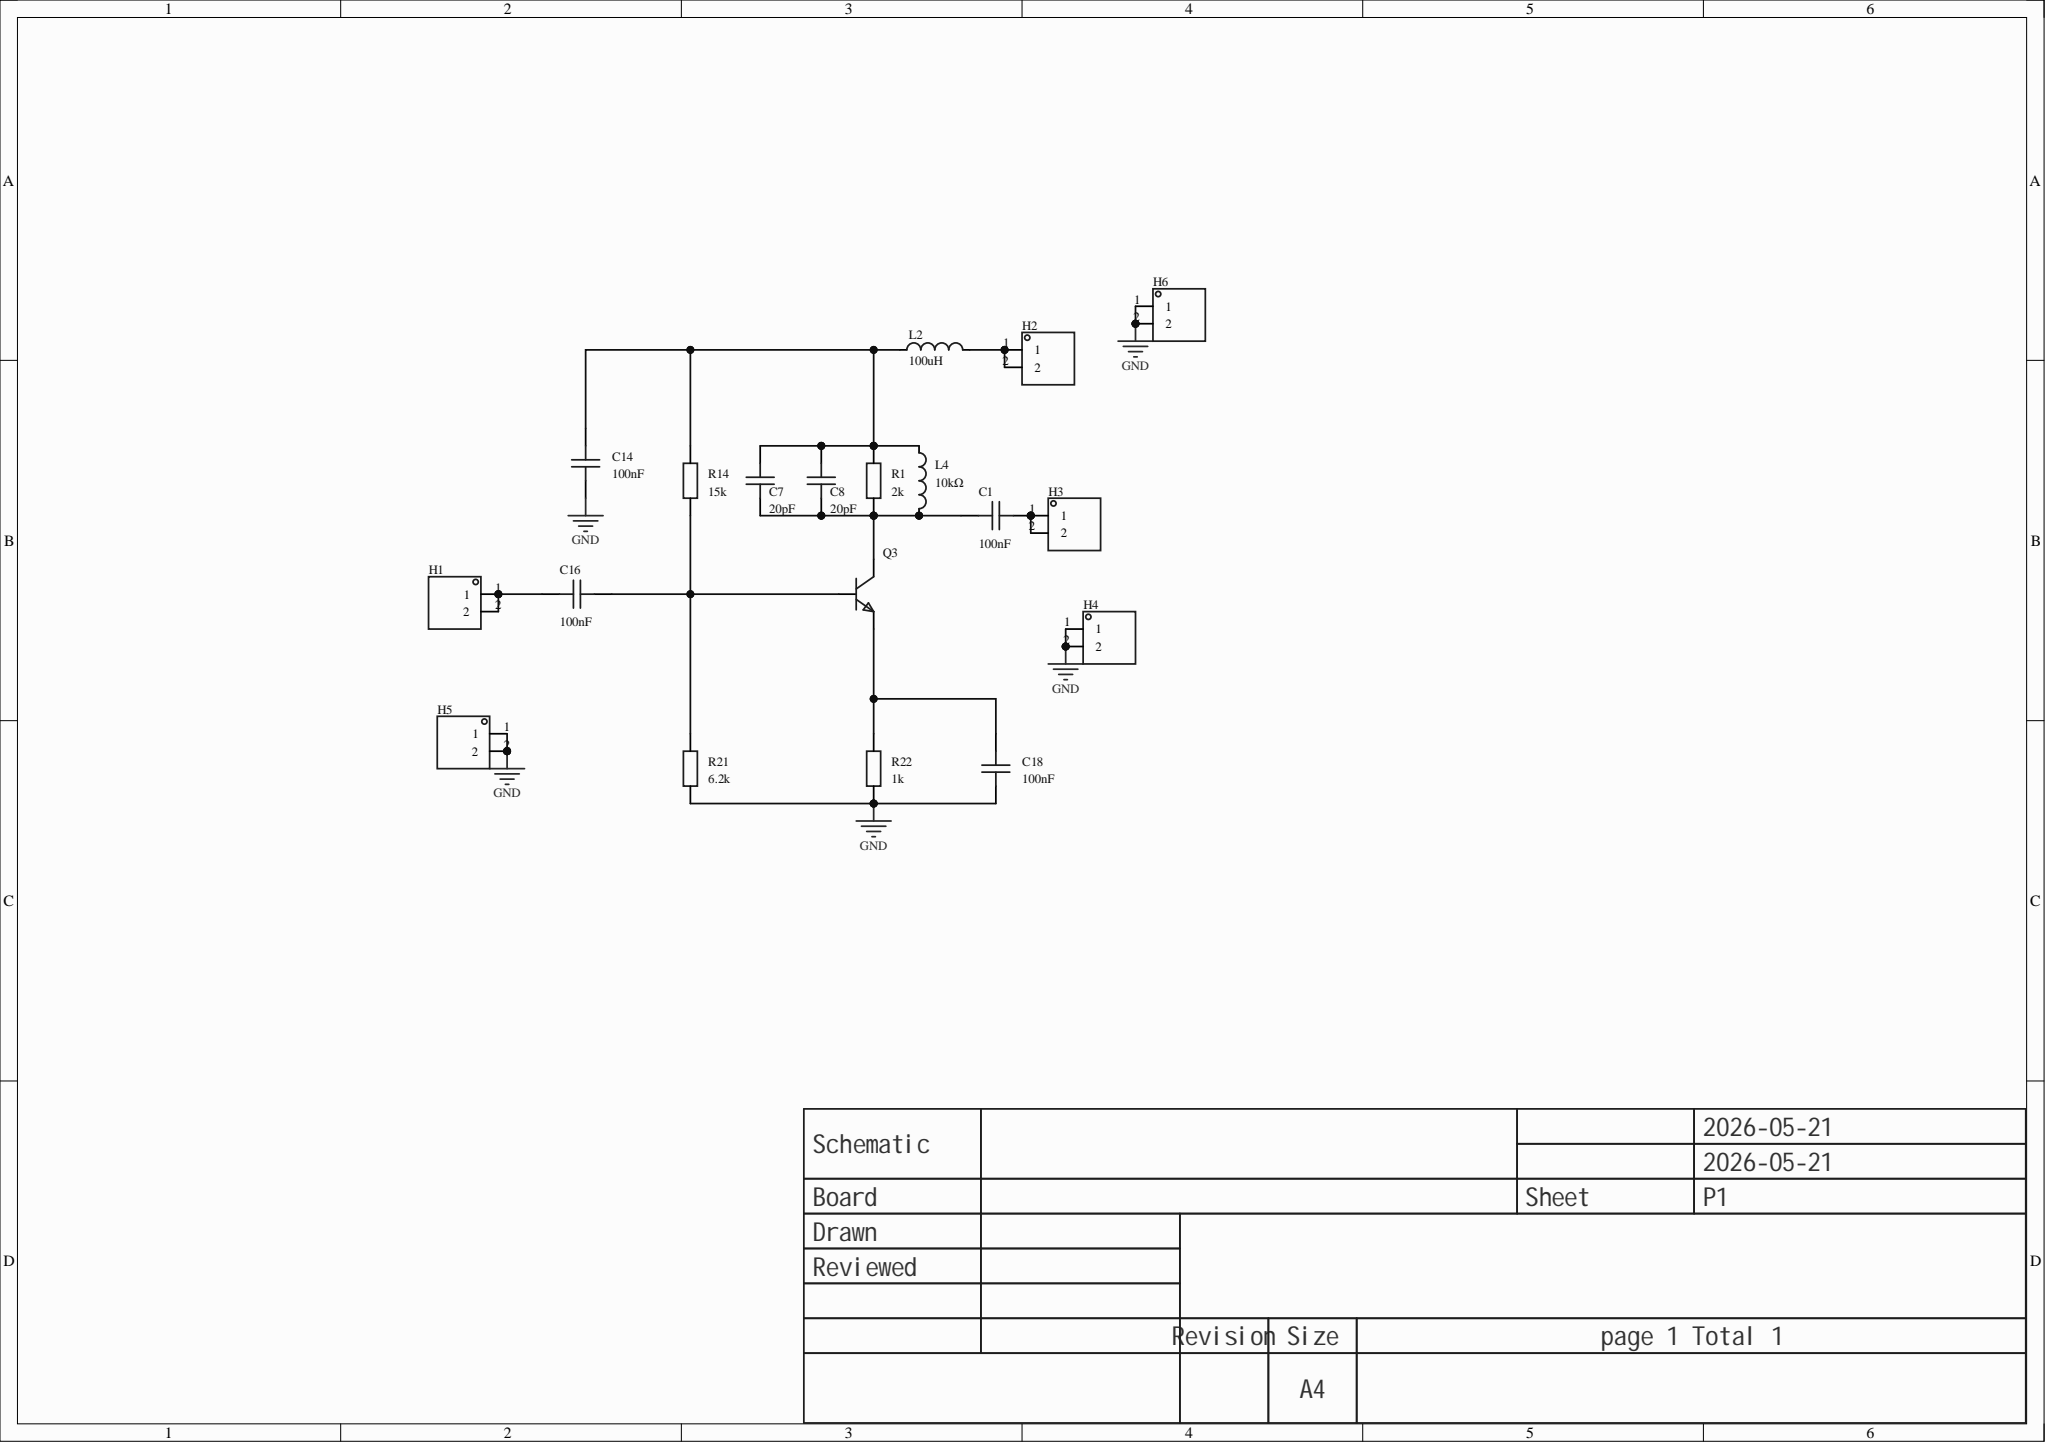Circuit board | Altium Designer | 19 parts | 8 nets
Bill of materials:
Comment,Description,Designator,Footprint,LibRef,Quantity
"100nF","","C1, C14, C16, C18","C0805","CAP_0603","4"
"20pF","","C7, C8","C0805","CAP_0603","2"
"","","H1, H2, H3, H4, H5, H6","HDR-TH_2P-P2.54-V-M-1","HDR-M_2.54_1x2P","6"
"100uH","SMD wire-wound inductor","L2","IND-SMD_L5.8-W5.2","INDUCTOR_CD54","1"
"10kΩ","","L4","Res_1/4W","Res_AXIAL-1/4W","1"
"","","Q3","S8050_TO_92","S8050_TO_NPN","1"
"2k","","R1","R0805","Res_0603","1"
"15k","","R14","R0805","Res_0603","1"
"6.2k","","R21","R0805","Res_0603","1"
"1k","","R22","R0805","Res_0603","1"
Netlist (Protel format):
[
C1
C0805
100nF



]
[
C7
C0805
20pF



]
[
C8
C0805
20pF



]
[
C14
C0805
100nF



]
[
C16
C0805
100nF



]
[
C18
C0805
100nF



]
[
H1
HDR-TH_2P-P2.54-V-M-1




]
[
H2
HDR-TH_2P-P2.54-V-M-1




]
[
H3
HDR-TH_2P-P2.54-V-M-1




]
[
H4
HDR-TH_2P-P2.54-V-M-1




]
[
H5
HDR-TH_2P-P2.54-V-M-1




]
[
H6
HDR-TH_2P-P2.54-V-M-1




]
[
L2
IND-SMD_L5.8-W5.2
100uH



]
[
L4
Res_1/4W
10kΩ



]
[
Q3
S8050_TO_92




]
[
R1
R0805
2k



]
[
R14
R0805
15k



]
[
R21
R0805
6.2k



]
[
R22
R0805
1k



]
(
NetH2_1
H2-1
H2-2
L2-2
)
(
NetC18_1
C18-1
Q3-1
R22-2
)
(
NetC16_2
C16-2
H1-1
H1-2
)
(
NetC16_1
C16-1
Q3-2
R14-1
R21-2
)
(
NetC7_2
C7-2
C8-2
C14-2
L2-1
L4-2
R1-2
R14-2
)
(
NetC1_2
C1-2
H3-1
H3-2
)
(
NetC1_1
C1-1
C7-1
C8-1
L4-1
Q3-3
R1-1
)
(
GND
C14-1
C18-2
H4-1
H4-2
H5-1
H5-2
H6-1
H6-2
R21-1
R22-1
)